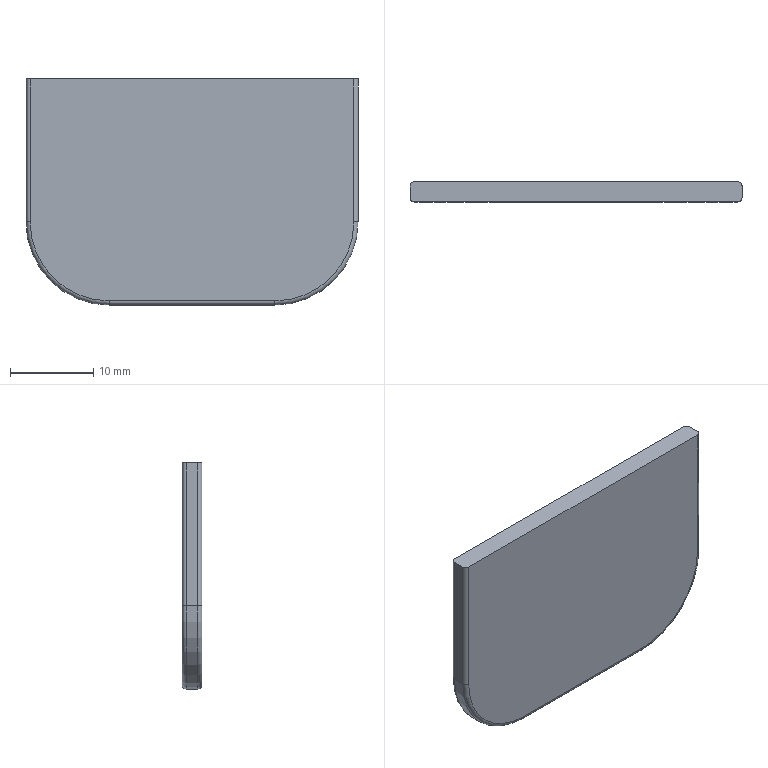Part | STEP file | 1 solid | 18 faces | box 39.94 x 2.4 x 27.2 mm | volume 2495 mm3 | cylinder 8 | plane 6 | torus 4 | commonest cylinder face diameters 1 x6 20 x2
STEP:
#1=CARTESIAN_POINT('',(0.,0.,0.));
#2=DIRECTION('',(0.,0.,1.));
#3=DIRECTION('',(1.,0.,0.));
#4=AXIS2_PLACEMENT_3D('',#1,#2,#3);
#5=CARTESIAN_POINT('',(1352.247,433.78,23.879));
#6=VERTEX_POINT('',#5);
#7=CARTESIAN_POINT('',(1352.247,435.18,23.879));
#8=VERTEX_POINT('',#7);
#9=CARTESIAN_POINT('',(1352.247,-3550.289,23.879));
#10=DIRECTION('',(0.,1.,0.));
#11=VECTOR('',#10,1.);
#12=LINE('',#9,#11);
#13=CARTESIAN_POINT('',(1352.247,433.23,0.979));
#14=DIRECTION('',(1.,0.,0.));
#15=DIRECTION('',(0.,0.,-1.));
#16=AXIS2_PLACEMENT_3D('',#13,#14,#15);
#17=PLANE('',#16);
#18=CARTESIAN_POINT('',(-22.9,-3983.519));
#19=DIRECTION('',(0.,1.));
#20=VECTOR('',#19,1.);
#21=LINE('',#18,#20);
#22=(GEOMETRIC_REPRESENTATION_CONTEXT(2)PARAMETRIC_REPRESENTATION_CONTEXT()REPRESENTATION_CONTEXT('',''));
#23=DEFINITIONAL_REPRESENTATION('',(#21),#22);
#24=PCURVE('',#17,#23);
#25=CARTESIAN_POINT('',(18395.161,-3550.289,23.879));
#26=DIRECTION('',(0.,0.,1.));
#27=DIRECTION('',(1.,0.,0.));
#28=AXIS2_PLACEMENT_3D('',#25,#26,#27);
#29=PLANE('',#28);
#30=CARTESIAN_POINT('',(-17042.914,0.));
#31=DIRECTION('',(0.,1.));
#32=VECTOR('',#31,1.);
#33=LINE('',#30,#32);
#34=(GEOMETRIC_REPRESENTATION_CONTEXT(2)PARAMETRIC_REPRESENTATION_CONTEXT()REPRESENTATION_CONTEXT('',''));
#35=DEFINITIONAL_REPRESENTATION('',(#33),#34);
#36=PCURVE('',#29,#35);
#37=SURFACE_CURVE('',#12,(#24,#36),.PCURVE_S1.);
#38=EDGE_CURVE('',#6,#8,#37,.T.);
#39=ORIENTED_EDGE('',*,*,#38,.F.);
#40=CARTESIAN_POINT('',(1352.247,433.78,6.679));
#41=VERTEX_POINT('',#40);
#42=CARTESIAN_POINT('',(1352.247,433.78,0.979));
#43=DIRECTION('',(0.,0.,-1.));
#44=VECTOR('',#43,1.);
#45=LINE('',#42,#44);
#46=CARTESIAN_POINT('',(0.,0.55));
#47=DIRECTION('',(1.,0.));
#48=VECTOR('',#47,1.);
#49=LINE('',#46,#48);
#50=(GEOMETRIC_REPRESENTATION_CONTEXT(2)PARAMETRIC_REPRESENTATION_CONTEXT()REPRESENTATION_CONTEXT('',''));
#51=DEFINITIONAL_REPRESENTATION('',(#49),#50);
#52=PCURVE('',#17,#51);
#53=CARTESIAN_POINT('',(1351.747,433.78,0.979));
#54=DIRECTION('',(0.,0.,1.));
#55=DIRECTION('',(1.,0.,0.));
#56=AXIS2_PLACEMENT_3D('',#53,#54,#55);
#57=CYLINDRICAL_SURFACE('',#56,0.5);
#58=CARTESIAN_POINT('',(6.283,0.));
#59=DIRECTION('',(0.,-1.));
#60=VECTOR('',#59,1.);
#61=LINE('',#58,#60);
#62=(GEOMETRIC_REPRESENTATION_CONTEXT(2)PARAMETRIC_REPRESENTATION_CONTEXT()REPRESENTATION_CONTEXT('',''));
#63=DEFINITIONAL_REPRESENTATION('',(#61),#62);
#64=PCURVE('',#57,#63);
#65=SURFACE_CURVE('',#45,(#52,#64),.PCURVE_S1.);
#66=EDGE_CURVE('',#6,#41,#65,.T.);
#67=ORIENTED_EDGE('',*,*,#66,.T.);
#68=CARTESIAN_POINT('',(1352.247,435.18,6.679));
#69=VERTEX_POINT('',#68);
#70=CARTESIAN_POINT('',(1352.247,435.68,6.679));
#71=DIRECTION('',(0.,1.,0.));
#72=VECTOR('',#71,1.);
#73=LINE('',#70,#72);
#74=CARTESIAN_POINT('',(-5.7,2.45));
#75=DIRECTION('',(0.,1.));
#76=VECTOR('',#75,1.);
#77=LINE('',#74,#76);
#78=(GEOMETRIC_REPRESENTATION_CONTEXT(2)PARAMETRIC_REPRESENTATION_CONTEXT()REPRESENTATION_CONTEXT('',''));
#79=DEFINITIONAL_REPRESENTATION('',(#77),#78);
#80=PCURVE('',#17,#79);
#81=CARTESIAN_POINT('',(1342.247,433.23,6.679));
#82=DIRECTION('',(0.,1.,0.));
#83=DIRECTION('',(0.,0.,-1.));
#84=AXIS2_PLACEMENT_3D('',#81,#82,#83);
#85=CYLINDRICAL_SURFACE('',#84,10.);
#86=CARTESIAN_POINT('',(4.712,2.45));
#87=DIRECTION('',(0.,1.));
#88=VECTOR('',#87,1.);
#89=LINE('',#86,#88);
#90=(GEOMETRIC_REPRESENTATION_CONTEXT(2)PARAMETRIC_REPRESENTATION_CONTEXT()REPRESENTATION_CONTEXT('',''));
#91=DEFINITIONAL_REPRESENTATION('',(#89),#90);
#92=PCURVE('',#85,#91);
#93=SURFACE_CURVE('',#73,(#80,#92),.PCURVE_S1.);
#94=EDGE_CURVE('',#41,#69,#93,.T.);
#95=ORIENTED_EDGE('',*,*,#94,.T.);
#96=CARTESIAN_POINT('',(1352.247,435.18,0.979));
#97=DIRECTION('',(0.,0.,1.));
#98=VECTOR('',#97,1.);
#99=LINE('',#96,#98);
#100=CARTESIAN_POINT('',(0.,1.95));
#101=DIRECTION('',(-1.,0.));
#102=VECTOR('',#101,1.);
#103=LINE('',#100,#102);
#104=(GEOMETRIC_REPRESENTATION_CONTEXT(2)PARAMETRIC_REPRESENTATION_CONTEXT()REPRESENTATION_CONTEXT('',''));
#105=DEFINITIONAL_REPRESENTATION('',(#103),#104);
#106=PCURVE('',#17,#105);
#107=CARTESIAN_POINT('',(1351.747,435.18,0.979));
#108=DIRECTION('',(0.,0.,1.));
#109=DIRECTION('',(1.,0.,0.));
#110=AXIS2_PLACEMENT_3D('',#107,#108,#109);
#111=CYLINDRICAL_SURFACE('',#110,0.5);
#112=CARTESIAN_POINT('',(0.,0.));
#113=DIRECTION('',(0.,1.));
#114=VECTOR('',#113,1.);
#115=LINE('',#112,#114);
#116=(GEOMETRIC_REPRESENTATION_CONTEXT(2)PARAMETRIC_REPRESENTATION_CONTEXT()REPRESENTATION_CONTEXT('',''));
#117=DEFINITIONAL_REPRESENTATION('',(#115),#116);
#118=PCURVE('',#111,#117);
#119=SURFACE_CURVE('',#99,(#106,#118),.PCURVE_S1.);
#120=EDGE_CURVE('',#69,#8,#119,.T.);
#121=ORIENTED_EDGE('',*,*,#120,.T.);
#122=EDGE_LOOP('',(#39,#67,#95,#121));
#123=FACE_BOUND('',#122,.T.);
#124=ADVANCED_FACE('',(#123),#17,.T.);
#125=CARTESIAN_POINT('',(1351.747,435.68,23.879));
#126=VERTEX_POINT('',#125);
#127=CARTESIAN_POINT('',(1312.807,435.68,23.879));
#128=VERTEX_POINT('',#127);
#129=CARTESIAN_POINT('',(18395.161,435.68,23.879));
#130=DIRECTION('',(-1.,0.,0.));
#131=VECTOR('',#130,1.);
#132=LINE('',#129,#131);
#133=CARTESIAN_POINT('',(1352.277,435.68,0.979));
#134=DIRECTION('',(0.,1.,0.));
#135=DIRECTION('',(0.,0.,-1.));
#136=AXIS2_PLACEMENT_3D('',#133,#134,#135);
#137=PLANE('',#136);
#138=CARTESIAN_POINT('',(-22.9,-17042.884));
#139=DIRECTION('',(0.,1.));
#140=VECTOR('',#139,1.);
#141=LINE('',#138,#140);
#142=(GEOMETRIC_REPRESENTATION_CONTEXT(2)PARAMETRIC_REPRESENTATION_CONTEXT()REPRESENTATION_CONTEXT('',''));
#143=DEFINITIONAL_REPRESENTATION('',(#141),#142);
#144=PCURVE('',#137,#143);
#145=CARTESIAN_POINT('',(0.,3985.969));
#146=DIRECTION('',(-1.,0.));
#147=VECTOR('',#146,1.);
#148=LINE('',#145,#147);
#149=(GEOMETRIC_REPRESENTATION_CONTEXT(2)PARAMETRIC_REPRESENTATION_CONTEXT()REPRESENTATION_CONTEXT('',''));
#150=DEFINITIONAL_REPRESENTATION('',(#148),#149);
#151=PCURVE('',#29,#150);
#152=SURFACE_CURVE('',#132,(#144,#151),.PCURVE_S1.);
#153=EDGE_CURVE('',#126,#128,#152,.T.);
#154=ORIENTED_EDGE('',*,*,#153,.F.);
#155=CARTESIAN_POINT('',(1351.747,435.68,6.679));
#156=VERTEX_POINT('',#155);
#157=CARTESIAN_POINT('',(1351.747,435.68,0.979));
#158=DIRECTION('',(0.,0.,-1.));
#159=VECTOR('',#158,1.);
#160=LINE('',#157,#159);
#161=CARTESIAN_POINT('',(0.,0.53));
#162=DIRECTION('',(1.,0.));
#163=VECTOR('',#162,1.);
#164=LINE('',#161,#163);
#165=(GEOMETRIC_REPRESENTATION_CONTEXT(2)PARAMETRIC_REPRESENTATION_CONTEXT()REPRESENTATION_CONTEXT('',''));
#166=DEFINITIONAL_REPRESENTATION('',(#164),#165);
#167=PCURVE('',#137,#166);
#168=CARTESIAN_POINT('',(1.571,0.));
#169=DIRECTION('',(0.,-1.));
#170=VECTOR('',#169,1.);
#171=LINE('',#168,#170);
#172=(GEOMETRIC_REPRESENTATION_CONTEXT(2)PARAMETRIC_REPRESENTATION_CONTEXT()REPRESENTATION_CONTEXT('',''));
#173=DEFINITIONAL_REPRESENTATION('',(#171),#172);
#174=PCURVE('',#111,#173);
#175=SURFACE_CURVE('',#160,(#167,#174),.PCURVE_S1.);
#176=EDGE_CURVE('',#126,#156,#175,.T.);
#177=ORIENTED_EDGE('',*,*,#176,.T.);
#178=CARTESIAN_POINT('',(1342.247,435.68,-2.821));
#179=VERTEX_POINT('',#178);
#180=CARTESIAN_POINT('',(1342.247,435.68,6.679));
#181=DIRECTION('',(0.,1.,0.));
#182=DIRECTION('',(0.,0.,1.));
#183=AXIS2_PLACEMENT_3D('',#180,#181,#182);
#184=CIRCLE('',#183,9.5);
#185=CARTESIAN_POINT('',(-5.7,10.03));
#186=DIRECTION('',(-1.,0.));
#187=AXIS2_PLACEMENT_2D('',#185,#186);
#188=CIRCLE('',#187,9.5);
#189=(GEOMETRIC_REPRESENTATION_CONTEXT(2)PARAMETRIC_REPRESENTATION_CONTEXT()REPRESENTATION_CONTEXT('',''));
#190=DEFINITIONAL_REPRESENTATION('',(#188),#189);
#191=PCURVE('',#137,#190);
#192=CARTESIAN_POINT('',(1342.247,435.18,6.679));
#193=DIRECTION('',(0.,1.,0.));
#194=DIRECTION('',(0.,0.,-1.));
#195=AXIS2_PLACEMENT_3D('',#192,#193,#194);
#196=TOROIDAL_SURFACE('',#195,9.5,0.5);
#197=CARTESIAN_POINT('',(3.142,1.571));
#198=DIRECTION('',(1.,0.));
#199=VECTOR('',#198,1.);
#200=LINE('',#197,#199);
#201=(GEOMETRIC_REPRESENTATION_CONTEXT(2)PARAMETRIC_REPRESENTATION_CONTEXT()REPRESENTATION_CONTEXT('',''));
#202=DEFINITIONAL_REPRESENTATION('',(#200),#201);
#203=PCURVE('',#196,#202);
#204=SURFACE_CURVE('',#184,(#191,#203),.PCURVE_S1.);
#205=EDGE_CURVE('',#156,#179,#204,.T.);
#206=ORIENTED_EDGE('',*,*,#205,.T.);
#207=CARTESIAN_POINT('',(1322.307,435.68,-2.821));
#208=VERTEX_POINT('',#207);
#209=CARTESIAN_POINT('',(1322.307,435.68,-2.821));
#210=DIRECTION('',(-1.,0.,0.));
#211=VECTOR('',#210,1.);
#212=LINE('',#209,#211);
#213=CARTESIAN_POINT('',(3.8,29.97));
#214=DIRECTION('',(0.,1.));
#215=VECTOR('',#214,1.);
#216=LINE('',#213,#215);
#217=(GEOMETRIC_REPRESENTATION_CONTEXT(2)PARAMETRIC_REPRESENTATION_CONTEXT()REPRESENTATION_CONTEXT('',''));
#218=DEFINITIONAL_REPRESENTATION('',(#216),#217);
#219=PCURVE('',#137,#218);
#220=CARTESIAN_POINT('',(1352.277,435.18,-2.821));
#221=DIRECTION('',(-1.,0.,0.));
#222=DIRECTION('',(0.,0.,1.));
#223=AXIS2_PLACEMENT_3D('',#220,#221,#222);
#224=CYLINDRICAL_SURFACE('',#223,0.5);
#225=CARTESIAN_POINT('',(1.571,29.97));
#226=DIRECTION('',(0.,1.));
#227=VECTOR('',#226,1.);
#228=LINE('',#225,#227);
#229=(GEOMETRIC_REPRESENTATION_CONTEXT(2)PARAMETRIC_REPRESENTATION_CONTEXT()REPRESENTATION_CONTEXT('',''));
#230=DEFINITIONAL_REPRESENTATION('',(#228),#229);
#231=PCURVE('',#224,#230);
#232=SURFACE_CURVE('',#212,(#219,#231),.PCURVE_S1.);
#233=EDGE_CURVE('',#179,#208,#232,.T.);
#234=ORIENTED_EDGE('',*,*,#233,.T.);
#235=CARTESIAN_POINT('',(1312.807,435.68,6.679));
#236=VERTEX_POINT('',#235);
#237=CARTESIAN_POINT('',(1322.307,435.68,6.679));
#238=DIRECTION('',(0.,1.,0.));
#239=DIRECTION('',(0.,0.,1.));
#240=AXIS2_PLACEMENT_3D('',#237,#238,#239);
#241=CIRCLE('',#240,9.5);
#242=CARTESIAN_POINT('',(-5.7,29.97));
#243=DIRECTION('',(-1.,0.));
#244=AXIS2_PLACEMENT_2D('',#242,#243);
#245=CIRCLE('',#244,9.5);
#246=(GEOMETRIC_REPRESENTATION_CONTEXT(2)PARAMETRIC_REPRESENTATION_CONTEXT()REPRESENTATION_CONTEXT('',''));
#247=DEFINITIONAL_REPRESENTATION('',(#245),#246);
#248=PCURVE('',#137,#247);
#249=CARTESIAN_POINT('',(1322.307,435.18,6.679));
#250=DIRECTION('',(0.,1.,0.));
#251=DIRECTION('',(0.,0.,-1.));
#252=AXIS2_PLACEMENT_3D('',#249,#250,#251);
#253=TOROIDAL_SURFACE('',#252,9.5,0.5);
#254=CARTESIAN_POINT('',(-3.142,1.571));
#255=DIRECTION('',(1.,0.));
#256=VECTOR('',#255,1.);
#257=LINE('',#254,#256);
#258=(GEOMETRIC_REPRESENTATION_CONTEXT(2)PARAMETRIC_REPRESENTATION_CONTEXT()REPRESENTATION_CONTEXT('',''));
#259=DEFINITIONAL_REPRESENTATION('',(#257),#258);
#260=PCURVE('',#253,#259);
#261=SURFACE_CURVE('',#241,(#248,#260),.PCURVE_S1.);
#262=EDGE_CURVE('',#208,#236,#261,.T.);
#263=ORIENTED_EDGE('',*,*,#262,.T.);
#264=CARTESIAN_POINT('',(1312.807,435.68,0.979));
#265=DIRECTION('',(0.,0.,1.));
#266=VECTOR('',#265,1.);
#267=LINE('',#264,#266);
#268=CARTESIAN_POINT('',(0.,39.47));
#269=DIRECTION('',(-1.,0.));
#270=VECTOR('',#269,1.);
#271=LINE('',#268,#270);
#272=(GEOMETRIC_REPRESENTATION_CONTEXT(2)PARAMETRIC_REPRESENTATION_CONTEXT()REPRESENTATION_CONTEXT('',''));
#273=DEFINITIONAL_REPRESENTATION('',(#271),#272);
#274=PCURVE('',#137,#273);
#275=CARTESIAN_POINT('',(1312.807,435.18,0.979));
#276=DIRECTION('',(0.,0.,1.));
#277=DIRECTION('',(1.,0.,0.));
#278=AXIS2_PLACEMENT_3D('',#275,#276,#277);
#279=CYLINDRICAL_SURFACE('',#278,0.5);
#280=CARTESIAN_POINT('',(1.571,0.));
#281=DIRECTION('',(0.,1.));
#282=VECTOR('',#281,1.);
#283=LINE('',#280,#282);
#284=(GEOMETRIC_REPRESENTATION_CONTEXT(2)PARAMETRIC_REPRESENTATION_CONTEXT()REPRESENTATION_CONTEXT('',''));
#285=DEFINITIONAL_REPRESENTATION('',(#283),#284);
#286=PCURVE('',#279,#285);
#287=SURFACE_CURVE('',#267,(#274,#286),.PCURVE_S1.);
#288=EDGE_CURVE('',#236,#128,#287,.T.);
#289=ORIENTED_EDGE('',*,*,#288,.T.);
#290=EDGE_LOOP('',(#154,#177,#206,#234,#263,#289));
#291=FACE_BOUND('',#290,.T.);
#292=ADVANCED_FACE('',(#291),#137,.T.);
#293=CARTESIAN_POINT('',(1312.307,435.18,6.679));
#294=VERTEX_POINT('',#293);
#295=CARTESIAN_POINT('',(1312.307,433.78,6.679));
#296=VERTEX_POINT('',#295);
#297=CARTESIAN_POINT('',(1312.307,433.28,6.679));
#298=DIRECTION('',(0.,-1.,0.));
#299=VECTOR('',#298,1.);
#300=LINE('',#297,#299);
#301=CARTESIAN_POINT('',(1312.307,435.73,0.979));
#302=DIRECTION('',(-1.,0.,0.));
#303=DIRECTION('',(0.,0.,1.));
#304=AXIS2_PLACEMENT_3D('',#301,#302,#303);
#305=PLANE('',#304);
#306=CARTESIAN_POINT('',(5.7,-2.45));
#307=DIRECTION('',(0.,-1.));
#308=VECTOR('',#307,1.);
#309=LINE('',#306,#308);
#310=(GEOMETRIC_REPRESENTATION_CONTEXT(2)PARAMETRIC_REPRESENTATION_CONTEXT()REPRESENTATION_CONTEXT('',''));
#311=DEFINITIONAL_REPRESENTATION('',(#309),#310);
#312=PCURVE('',#305,#311);
#313=CARTESIAN_POINT('',(1322.307,435.73,6.679));
#314=DIRECTION('',(0.,-1.,0.));
#315=DIRECTION('',(0.,0.,1.));
#316=AXIS2_PLACEMENT_3D('',#313,#314,#315);
#317=CYLINDRICAL_SURFACE('',#316,10.);
#318=CARTESIAN_POINT('',(1.571,2.45));
#319=DIRECTION('',(0.,1.));
#320=VECTOR('',#319,1.);
#321=LINE('',#318,#320);
#322=(GEOMETRIC_REPRESENTATION_CONTEXT(2)PARAMETRIC_REPRESENTATION_CONTEXT()REPRESENTATION_CONTEXT('',''));
#323=DEFINITIONAL_REPRESENTATION('',(#321),#322);
#324=PCURVE('',#317,#323);
#325=SURFACE_CURVE('',#300,(#312,#324),.PCURVE_S1.);
#326=EDGE_CURVE('',#294,#296,#325,.T.);
#327=ORIENTED_EDGE('',*,*,#326,.T.);
#328=CARTESIAN_POINT('',(1312.307,433.78,23.879));
#329=VERTEX_POINT('',#328);
#330=CARTESIAN_POINT('',(1312.307,433.78,0.979));
#331=DIRECTION('',(0.,0.,1.));
#332=VECTOR('',#331,1.);
#333=LINE('',#330,#332);
#334=CARTESIAN_POINT('',(0.,-1.95));
#335=DIRECTION('',(1.,0.));
#336=VECTOR('',#335,1.);
#337=LINE('',#334,#336);
#338=(GEOMETRIC_REPRESENTATION_CONTEXT(2)PARAMETRIC_REPRESENTATION_CONTEXT()REPRESENTATION_CONTEXT('',''));
#339=DEFINITIONAL_REPRESENTATION('',(#337),#338);
#340=PCURVE('',#305,#339);
#341=CARTESIAN_POINT('',(1312.807,433.78,0.979));
#342=DIRECTION('',(0.,0.,1.));
#343=DIRECTION('',(1.,0.,0.));
#344=AXIS2_PLACEMENT_3D('',#341,#342,#343);
#345=CYLINDRICAL_SURFACE('',#344,0.5);
#346=CARTESIAN_POINT('',(3.142,0.));
#347=DIRECTION('',(0.,1.));
#348=VECTOR('',#347,1.);
#349=LINE('',#346,#348);
#350=(GEOMETRIC_REPRESENTATION_CONTEXT(2)PARAMETRIC_REPRESENTATION_CONTEXT()REPRESENTATION_CONTEXT('',''));
#351=DEFINITIONAL_REPRESENTATION('',(#349),#350);
#352=PCURVE('',#345,#351);
#353=SURFACE_CURVE('',#333,(#340,#352),.PCURVE_S1.);
#354=EDGE_CURVE('',#296,#329,#353,.T.);
#355=ORIENTED_EDGE('',*,*,#354,.T.);
#356=CARTESIAN_POINT('',(1312.307,435.18,23.879));
#357=VERTEX_POINT('',#356);
#358=CARTESIAN_POINT('',(1312.307,-3550.289,23.879));
#359=DIRECTION('',(0.,-1.,0.));
#360=VECTOR('',#359,1.);
#361=LINE('',#358,#360);
#362=CARTESIAN_POINT('',(22.9,-3986.019));
#363=DIRECTION('',(0.,-1.));
#364=VECTOR('',#363,1.);
#365=LINE('',#362,#364);
#366=(GEOMETRIC_REPRESENTATION_CONTEXT(2)PARAMETRIC_REPRESENTATION_CONTEXT()REPRESENTATION_CONTEXT('',''));
#367=DEFINITIONAL_REPRESENTATION('',(#365),#366);
#368=PCURVE('',#305,#367);
#369=CARTESIAN_POINT('',(-17082.854,0.));
#370=DIRECTION('',(0.,-1.));
#371=VECTOR('',#370,1.);
#372=LINE('',#369,#371);
#373=(GEOMETRIC_REPRESENTATION_CONTEXT(2)PARAMETRIC_REPRESENTATION_CONTEXT()REPRESENTATION_CONTEXT('',''));
#374=DEFINITIONAL_REPRESENTATION('',(#372),#373);
#375=PCURVE('',#29,#374);
#376=SURFACE_CURVE('',#361,(#368,#375),.PCURVE_S1.);
#377=EDGE_CURVE('',#357,#329,#376,.T.);
#378=ORIENTED_EDGE('',*,*,#377,.F.);
#379=CARTESIAN_POINT('',(1312.307,435.18,0.979));
#380=DIRECTION('',(0.,0.,-1.));
#381=VECTOR('',#380,1.);
#382=LINE('',#379,#381);
#383=CARTESIAN_POINT('',(0.,-0.55));
#384=DIRECTION('',(-1.,0.));
#385=VECTOR('',#384,1.);
#386=LINE('',#383,#385);
#387=(GEOMETRIC_REPRESENTATION_CONTEXT(2)PARAMETRIC_REPRESENTATION_CONTEXT()REPRESENTATION_CONTEXT('',''));
#388=DEFINITIONAL_REPRESENTATION('',(#386),#387);
#389=PCURVE('',#305,#388);
#390=CARTESIAN_POINT('',(3.142,0.));
#391=DIRECTION('',(0.,-1.));
#392=VECTOR('',#391,1.);
#393=LINE('',#390,#392);
#394=(GEOMETRIC_REPRESENTATION_CONTEXT(2)PARAMETRIC_REPRESENTATION_CONTEXT()REPRESENTATION_CONTEXT('',''));
#395=DEFINITIONAL_REPRESENTATION('',(#393),#394);
#396=PCURVE('',#279,#395);
#397=SURFACE_CURVE('',#382,(#389,#396),.PCURVE_S1.);
#398=EDGE_CURVE('',#357,#294,#397,.T.);
#399=ORIENTED_EDGE('',*,*,#398,.T.);
#400=EDGE_LOOP('',(#327,#355,#378,#399));
#401=FACE_BOUND('',#400,.T.);
#402=ADVANCED_FACE('',(#401),#305,.T.);
#403=CARTESIAN_POINT('',(1312.807,433.28,23.879));
#404=VERTEX_POINT('',#403);
#405=CARTESIAN_POINT('',(1351.747,433.28,23.879));
#406=VERTEX_POINT('',#405);
#407=CARTESIAN_POINT('',(18395.161,433.28,23.879));
#408=DIRECTION('',(1.,0.,0.));
#409=VECTOR('',#408,1.);
#410=LINE('',#407,#409);
#411=CARTESIAN_POINT('',(1312.277,433.28,0.979));
#412=DIRECTION('',(0.,-1.,0.));
#413=DIRECTION('',(0.,0.,1.));
#414=AXIS2_PLACEMENT_3D('',#411,#412,#413);
#415=PLANE('',#414);
#416=CARTESIAN_POINT('',(22.9,-17082.884));
#417=DIRECTION('',(0.,-1.));
#418=VECTOR('',#417,1.);
#419=LINE('',#416,#418);
#420=(GEOMETRIC_REPRESENTATION_CONTEXT(2)PARAMETRIC_REPRESENTATION_CONTEXT()REPRESENTATION_CONTEXT('',''));
#421=DEFINITIONAL_REPRESENTATION('',(#419),#420);
#422=PCURVE('',#415,#421);
#423=CARTESIAN_POINT('',(0.,3983.569));
#424=DIRECTION('',(1.,0.));
#425=VECTOR('',#424,1.);
#426=LINE('',#423,#425);
#427=(GEOMETRIC_REPRESENTATION_CONTEXT(2)PARAMETRIC_REPRESENTATION_CONTEXT()REPRESENTATION_CONTEXT('',''));
#428=DEFINITIONAL_REPRESENTATION('',(#426),#427);
#429=PCURVE('',#29,#428);
#430=SURFACE_CURVE('',#410,(#422,#429),.PCURVE_S1.);
#431=EDGE_CURVE('',#404,#406,#430,.T.);
#432=ORIENTED_EDGE('',*,*,#431,.F.);
#433=CARTESIAN_POINT('',(1312.807,433.28,6.679));
#434=VERTEX_POINT('',#433);
#435=CARTESIAN_POINT('',(1312.807,433.28,0.979));
#436=DIRECTION('',(0.,0.,-1.));
#437=VECTOR('',#436,1.);
#438=LINE('',#435,#437);
#439=CARTESIAN_POINT('',(0.,-0.53));
#440=DIRECTION('',(-1.,0.));
#441=VECTOR('',#440,1.);
#442=LINE('',#439,#441);
#443=(GEOMETRIC_REPRESENTATION_CONTEXT(2)PARAMETRIC_REPRESENTATION_CONTEXT()REPRESENTATION_CONTEXT('',''));
#444=DEFINITIONAL_REPRESENTATION('',(#442),#443);
#445=PCURVE('',#415,#444);
#446=CARTESIAN_POINT('',(4.712,0.));
#447=DIRECTION('',(0.,-1.));
#448=VECTOR('',#447,1.);
#449=LINE('',#446,#448);
#450=(GEOMETRIC_REPRESENTATION_CONTEXT(2)PARAMETRIC_REPRESENTATION_CONTEXT()REPRESENTATION_CONTEXT('',''));
#451=DEFINITIONAL_REPRESENTATION('',(#449),#450);
#452=PCURVE('',#345,#451);
#453=SURFACE_CURVE('',#438,(#445,#452),.PCURVE_S1.);
#454=EDGE_CURVE('',#404,#434,#453,.T.);
#455=ORIENTED_EDGE('',*,*,#454,.T.);
#456=CARTESIAN_POINT('',(1322.307,433.28,-2.821));
#457=VERTEX_POINT('',#456);
#458=CARTESIAN_POINT('',(1322.307,433.28,6.679));
#459=DIRECTION('',(0.,-1.,0.));
#460=DIRECTION('',(0.,0.,-1.));
#461=AXIS2_PLACEMENT_3D('',#458,#459,#460);
#462=CIRCLE('',#461,9.5);
#463=CARTESIAN_POINT('',(5.7,-10.03));
#464=DIRECTION('',(-1.,0.));
#465=AXIS2_PLACEMENT_2D('',#463,#464);
#466=CIRCLE('',#465,9.5);
#467=(GEOMETRIC_REPRESENTATION_CONTEXT(2)PARAMETRIC_REPRESENTATION_CONTEXT()REPRESENTATION_CONTEXT('',''));
#468=DEFINITIONAL_REPRESENTATION('',(#466),#467);
#469=PCURVE('',#415,#468);
#470=CARTESIAN_POINT('',(1322.307,433.78,6.679));
#471=DIRECTION('',(0.,-1.,0.));
#472=DIRECTION('',(0.,0.,1.));
#473=AXIS2_PLACEMENT_3D('',#470,#471,#472);
#474=TOROIDAL_SURFACE('',#473,9.5,0.5);
#475=CARTESIAN_POINT('',(-3.142,1.571));
#476=DIRECTION('',(1.,0.));
#477=VECTOR('',#476,1.);
#478=LINE('',#475,#477);
#479=(GEOMETRIC_REPRESENTATION_CONTEXT(2)PARAMETRIC_REPRESENTATION_CONTEXT()REPRESENTATION_CONTEXT('',''));
#480=DEFINITIONAL_REPRESENTATION('',(#478),#479);
#481=PCURVE('',#474,#480);
#482=SURFACE_CURVE('',#462,(#469,#481),.PCURVE_S1.);
#483=EDGE_CURVE('',#434,#457,#482,.T.);
#484=ORIENTED_EDGE('',*,*,#483,.T.);
#485=CARTESIAN_POINT('',(1342.247,433.28,-2.821));
#486=VERTEX_POINT('',#485);
#487=CARTESIAN_POINT('',(1342.247,433.28,-2.821));
#488=DIRECTION('',(1.,0.,0.));
#489=VECTOR('',#488,1.);
#490=LINE('',#487,#489);
#491=CARTESIAN_POINT('',(-3.8,-29.97));
#492=DIRECTION('',(0.,-1.));
#493=VECTOR('',#492,1.);
#494=LINE('',#491,#493);
#495=(GEOMETRIC_REPRESENTATION_CONTEXT(2)PARAMETRIC_REPRESENTATION_CONTEXT()REPRESENTATION_CONTEXT('',''));
#496=DEFINITIONAL_REPRESENTATION('',(#494),#495);
#497=PCURVE('',#415,#496);
#498=CARTESIAN_POINT('',(1312.277,433.78,-2.821));
#499=DIRECTION('',(1.,0.,0.));
#500=DIRECTION('',(0.,0.,-1.));
#501=AXIS2_PLACEMENT_3D('',#498,#499,#500);
#502=CYLINDRICAL_SURFACE('',#501,0.5);
#503=CARTESIAN_POINT('',(4.712,29.97));
#504=DIRECTION('',(0.,1.));
#505=VECTOR('',#504,1.);
#506=LINE('',#503,#505);
#507=(GEOMETRIC_REPRESENTATION_CONTEXT(2)PARAMETRIC_REPRESENTATION_CONTEXT()REPRESENTATION_CONTEXT('',''));
#508=DEFINITIONAL_REPRESENTATION('',(#506),#507);
#509=PCURVE('',#502,#508);
#510=SURFACE_CURVE('',#490,(#497,#509),.PCURVE_S1.);
#511=EDGE_CURVE('',#457,#486,#510,.T.);
#512=ORIENTED_EDGE('',*,*,#511,.T.);
#513=CARTESIAN_POINT('',(1351.747,433.28,6.679));
#514=VERTEX_POINT('',#513);
#515=CARTESIAN_POINT('',(1342.247,433.28,6.679));
#516=DIRECTION('',(0.,-1.,0.));
#517=DIRECTION('',(0.,0.,-1.));
#518=AXIS2_PLACEMENT_3D('',#515,#516,#517);
#519=CIRCLE('',#518,9.5);
#520=CARTESIAN_POINT('',(5.7,-29.97));
#521=DIRECTION('',(-1.,0.));
#522=AXIS2_PLACEMENT_2D('',#520,#521);
#523=CIRCLE('',#522,9.5);
#524=(GEOMETRIC_REPRESENTATION_CONTEXT(2)PARAMETRIC_REPRESENTATION_CONTEXT()REPRESENTATION_CONTEXT('',''));
#525=DEFINITIONAL_REPRESENTATION('',(#523),#524);
#526=PCURVE('',#415,#525);
#527=CARTESIAN_POINT('',(1342.247,433.78,6.679));
#528=DIRECTION('',(0.,-1.,0.));
#529=DIRECTION('',(0.,0.,1.));
#530=AXIS2_PLACEMENT_3D('',#527,#528,#529);
#531=TOROIDAL_SURFACE('',#530,9.5,0.5);
#532=CARTESIAN_POINT('',(3.142,1.571));
#533=DIRECTION('',(1.,0.));
#534=VECTOR('',#533,1.);
#535=LINE('',#532,#534);
#536=(GEOMETRIC_REPRESENTATION_CONTEXT(2)PARAMETRIC_REPRESENTATION_CONTEXT()REPRESENTATION_CONTEXT('',''));
#537=DEFINITIONAL_REPRESENTATION('',(#535),#536);
#538=PCURVE('',#531,#537);
#539=SURFACE_CURVE('',#519,(#526,#538),.PCURVE_S1.);
#540=EDGE_CURVE('',#486,#514,#539,.T.);
#541=ORIENTED_EDGE('',*,*,#540,.T.);
#542=CARTESIAN_POINT('',(1351.747,433.28,0.979));
#543=DIRECTION('',(0.,0.,1.));
#544=VECTOR('',#543,1.);
#545=LINE('',#542,#544);
#546=CARTESIAN_POINT('',(0.,-39.47));
#547=DIRECTION('',(1.,0.));
#548=VECTOR('',#547,1.);
#549=LINE('',#546,#548);
#550=(GEOMETRIC_REPRESENTATION_CONTEXT(2)PARAMETRIC_REPRESENTATION_CONTEXT()REPRESENTATION_CONTEXT('',''));
#551=DEFINITIONAL_REPRESENTATION('',(#549),#550);
#552=PCURVE('',#415,#551);
#553=CARTESIAN_POINT('',(4.712,0.));
#554=DIRECTION('',(0.,1.));
#555=VECTOR('',#554,1.);
#556=LINE('',#553,#555);
#557=(GEOMETRIC_REPRESENTATION_CONTEXT(2)PARAMETRIC_REPRESENTATION_CONTEXT()REPRESENTATION_CONTEXT('',''));
#558=DEFINITIONAL_REPRESENTATION('',(#556),#557);
#559=PCURVE('',#57,#558);
#560=SURFACE_CURVE('',#545,(#552,#559),.PCURVE_S1.);
#561=EDGE_CURVE('',#514,#406,#560,.T.);
#562=ORIENTED_EDGE('',*,*,#561,.T.);
#563=EDGE_LOOP('',(#432,#455,#484,#512,#541,#562));
#564=FACE_BOUND('',#563,.T.);
#565=ADVANCED_FACE('',(#564),#415,.T.);
#566=CARTESIAN_POINT('',(1342.247,435.18,-3.321));
#567=VERTEX_POINT('',#566);
#568=CARTESIAN_POINT('',(1342.247,433.78,-3.321));
#569=VERTEX_POINT('',#568);
#570=CARTESIAN_POINT('',(1342.247,433.28,-3.321));
#571=DIRECTION('',(0.,-1.,0.));
#572=VECTOR('',#571,1.);
#573=LINE('',#570,#572);
#574=CARTESIAN_POINT('',(1359.213,511.68,-3.321));
#575=DIRECTION('',(0.,0.,-1.));
#576=DIRECTION('',(-1.,0.,0.));
#577=AXIS2_PLACEMENT_3D('',#574,#575,#576);
#578=PLANE('',#577);
#579=CARTESIAN_POINT('',(16.966,-78.4));
#580=DIRECTION('',(0.,-1.));
#581=VECTOR('',#580,1.);
#582=LINE('',#579,#581);
#583=(GEOMETRIC_REPRESENTATION_CONTEXT(2)PARAMETRIC_REPRESENTATION_CONTEXT()REPRESENTATION_CONTEXT('',''));
#584=DEFINITIONAL_REPRESENTATION('',(#582),#583);
#585=PCURVE('',#578,#584);
#586=CARTESIAN_POINT('',(6.283,0.05));
#587=DIRECTION('',(0.,-1.));
#588=VECTOR('',#587,1.);
#589=LINE('',#586,#588);
#590=(GEOMETRIC_REPRESENTATION_CONTEXT(2)PARAMETRIC_REPRESENTATION_CONTEXT()REPRESENTATION_CONTEXT('',''));
#591=DEFINITIONAL_REPRESENTATION('',(#589),#590);
#592=PCURVE('',#85,#591);
#593=SURFACE_CURVE('',#573,(#585,#592),.PCURVE_S1.);
#594=EDGE_CURVE('',#567,#569,#593,.T.);
#595=ORIENTED_EDGE('',*,*,#594,.T.);
#596=CARTESIAN_POINT('',(1322.307,433.78,-3.321));
#597=VERTEX_POINT('',#596);
#598=CARTESIAN_POINT('',(1322.307,433.78,-3.321));
#599=DIRECTION('',(-1.,0.,0.));
#600=VECTOR('',#599,1.);
#601=LINE('',#598,#600);
#602=CARTESIAN_POINT('',(36.906,-77.9));
#603=DIRECTION('',(1.,0.));
#604=VECTOR('',#603,1.);
#605=LINE('',#602,#604);
#606=(GEOMETRIC_REPRESENTATION_CONTEXT(2)PARAMETRIC_REPRESENTATION_CONTEXT()REPRESENTATION_CONTEXT('',''));
#607=DEFINITIONAL_REPRESENTATION('',(#605),#606);
#608=PCURVE('',#578,#607);
#609=CARTESIAN_POINT('',(6.283,10.03));
#610=DIRECTION('',(0.,-1.));
#611=VECTOR('',#610,1.);
#612=LINE('',#609,#611);
#613=(GEOMETRIC_REPRESENTATION_CONTEXT(2)PARAMETRIC_REPRESENTATION_CONTEXT()REPRESENTATION_CONTEXT('',''));
#614=DEFINITIONAL_REPRESENTATION('',(#612),#613);
#615=PCURVE('',#502,#614);
#616=SURFACE_CURVE('',#601,(#608,#615),.PCURVE_S1.);
#617=EDGE_CURVE('',#569,#597,#616,.T.);
#618=ORIENTED_EDGE('',*,*,#617,.T.);
#619=CARTESIAN_POINT('',(1322.307,435.18,-3.321));
#620=VERTEX_POINT('',#619);
#621=CARTESIAN_POINT('',(1322.307,435.68,-3.321));
#622=DIRECTION('',(0.,1.,0.));
#623=VECTOR('',#622,1.);
#624=LINE('',#621,#623);
#625=CARTESIAN_POINT('',(36.906,-76.));
#626=DIRECTION('',(0.,1.));
#627=VECTOR('',#626,1.);
#628=LINE('',#625,#627);
#629=(GEOMETRIC_REPRESENTATION_CONTEXT(2)PARAMETRIC_REPRESENTATION_CONTEXT()REPRESENTATION_CONTEXT('',''));
#630=DEFINITIONAL_REPRESENTATION('',(#628),#629);
#631=PCURVE('',#578,#630);
#632=CARTESIAN_POINT('',(3.142,0.05));
#633=DIRECTION('',(0.,-1.));
#634=VECTOR('',#633,1.);
#635=LINE('',#632,#634);
#636=(GEOMETRIC_REPRESENTATION_CONTEXT(2)PARAMETRIC_REPRESENTATION_CONTEXT()REPRESENTATION_CONTEXT('',''));
#637=DEFINITIONAL_REPRESENTATION('',(#635),#636);
#638=PCURVE('',#317,#637);
#639=SURFACE_CURVE('',#624,(#631,#638),.PCURVE_S1.);
#640=EDGE_CURVE('',#597,#620,#639,.T.);
#641=ORIENTED_EDGE('',*,*,#640,.T.);
#642=CARTESIAN_POINT('',(1342.247,435.18,-3.321));
#643=DIRECTION('',(1.,0.,0.));
#644=VECTOR('',#643,1.);
#645=LINE('',#642,#644);
#646=CARTESIAN_POINT('',(16.966,-76.5));
#647=DIRECTION('',(-1.,0.));
#648=VECTOR('',#647,1.);
#649=LINE('',#646,#648);
#650=(GEOMETRIC_REPRESENTATION_CONTEXT(2)PARAMETRIC_REPRESENTATION_CONTEXT()REPRESENTATION_CONTEXT('',''));
#651=DEFINITIONAL_REPRESENTATION('',(#649),#650);
#652=PCURVE('',#578,#651);
#653=CARTESIAN_POINT('',(3.142,10.03));
#654=DIRECTION('',(0.,-1.));
#655=VECTOR('',#654,1.);
#656=LINE('',#653,#655);
#657=(GEOMETRIC_REPRESENTATION_CONTEXT(2)PARAMETRIC_REPRESENTATION_CONTEXT()REPRESENTATION_CONTEXT('',''));
#658=DEFINITIONAL_REPRESENTATION('',(#656),#657);
#659=PCURVE('',#224,#658);
#660=SURFACE_CURVE('',#645,(#652,#659),.PCURVE_S1.);
#661=EDGE_CURVE('',#620,#567,#660,.T.);
#662=ORIENTED_EDGE('',*,*,#661,.T.);
#663=EDGE_LOOP('',(#595,#618,#641,#662));
#664=FACE_BOUND('',#663,.T.);
#665=ADVANCED_FACE('',(#664),#578,.T.);
#666=ORIENTED_EDGE('',*,*,#377,.T.);
#667=CARTESIAN_POINT('',(1312.807,433.78,23.879));
#668=DIRECTION('',(0.,0.,1.));
#669=DIRECTION('',(-1.,0.,0.));
#670=AXIS2_PLACEMENT_3D('',#667,#668,#669);
#671=CIRCLE('',#670,0.5);
#672=CARTESIAN_POINT('',(-17082.354,3984.069));
#673=DIRECTION('',(-1.,0.));
#674=AXIS2_PLACEMENT_2D('',#672,#673);
#675=CIRCLE('',#674,0.5);
#676=(GEOMETRIC_REPRESENTATION_CONTEXT(2)PARAMETRIC_REPRESENTATION_CONTEXT()REPRESENTATION_CONTEXT('',''));
#677=DEFINITIONAL_REPRESENTATION('',(#675),#676);
#678=PCURVE('',#29,#677);
#679=CARTESIAN_POINT('',(3.142,22.9));
#680=DIRECTION('',(1.,0.));
#681=VECTOR('',#680,1.);
#682=LINE('',#679,#681);
#683=(GEOMETRIC_REPRESENTATION_CONTEXT(2)PARAMETRIC_REPRESENTATION_CONTEXT()REPRESENTATION_CONTEXT('',''));
#684=DEFINITIONAL_REPRESENTATION('',(#682),#683);
#685=PCURVE('',#345,#684);
#686=SURFACE_CURVE('',#671,(#678,#685),.PCURVE_S1.);
#687=EDGE_CURVE('',#329,#404,#686,.T.);
#688=ORIENTED_EDGE('',*,*,#687,.T.);
#689=ORIENTED_EDGE('',*,*,#431,.T.);
#690=CARTESIAN_POINT('',(1351.747,433.78,23.879));
#691=DIRECTION('',(0.,0.,1.));
#692=DIRECTION('',(-1.,0.,0.));
#693=AXIS2_PLACEMENT_3D('',#690,#691,#692);
#694=CIRCLE('',#693,0.5);
#695=CARTESIAN_POINT('',(-17043.414,3984.069));
#696=DIRECTION('',(-1.,0.));
#697=AXIS2_PLACEMENT_2D('',#695,#696);
#698=CIRCLE('',#697,0.5);
#699=(GEOMETRIC_REPRESENTATION_CONTEXT(2)PARAMETRIC_REPRESENTATION_CONTEXT()REPRESENTATION_CONTEXT('',''));
#700=DEFINITIONAL_REPRESENTATION('',(#698),#699);
#701=PCURVE('',#29,#700);
#702=CARTESIAN_POINT('',(3.142,22.9));
#703=DIRECTION('',(1.,0.));
#704=VECTOR('',#703,1.);
#705=LINE('',#702,#704);
#706=(GEOMETRIC_REPRESENTATION_CONTEXT(2)PARAMETRIC_REPRESENTATION_CONTEXT()REPRESENTATION_CONTEXT('',''));
#707=DEFINITIONAL_REPRESENTATION('',(#705),#706);
#708=PCURVE('',#57,#707);
#709=SURFACE_CURVE('',#694,(#701,#708),.PCURVE_S1.);
#710=EDGE_CURVE('',#406,#6,#709,.T.);
#711=ORIENTED_EDGE('',*,*,#710,.T.);
#712=ORIENTED_EDGE('',*,*,#38,.T.);
#713=CARTESIAN_POINT('',(1351.747,435.18,23.879));
#714=DIRECTION('',(0.,0.,1.));
#715=DIRECTION('',(-1.,0.,0.));
#716=AXIS2_PLACEMENT_3D('',#713,#714,#715);
#717=CIRCLE('',#716,0.5);
#718=CARTESIAN_POINT('',(-17043.414,3985.469));
#719=DIRECTION('',(-1.,0.));
#720=AXIS2_PLACEMENT_2D('',#718,#719);
#721=CIRCLE('',#720,0.5);
#722=(GEOMETRIC_REPRESENTATION_CONTEXT(2)PARAMETRIC_REPRESENTATION_CONTEXT()REPRESENTATION_CONTEXT('',''));
#723=DEFINITIONAL_REPRESENTATION('',(#721),#722);
#724=PCURVE('',#29,#723);
#725=CARTESIAN_POINT('',(-3.142,22.9));
#726=DIRECTION('',(1.,0.));
#727=VECTOR('',#726,1.);
#728=LINE('',#725,#727);
#729=(GEOMETRIC_REPRESENTATION_CONTEXT(2)PARAMETRIC_REPRESENTATION_CONTEXT()REPRESENTATION_CONTEXT('',''));
#730=DEFINITIONAL_REPRESENTATION('',(#728),#729);
#731=PCURVE('',#111,#730);
#732=SURFACE_CURVE('',#717,(#724,#731),.PCURVE_S1.);
#733=EDGE_CURVE('',#8,#126,#732,.T.);
#734=ORIENTED_EDGE('',*,*,#733,.T.);
#735=ORIENTED_EDGE('',*,*,#153,.T.);
#736=CARTESIAN_POINT('',(1312.807,435.18,23.879));
#737=DIRECTION('',(0.,0.,1.));
#738=DIRECTION('',(-1.,0.,0.));
#739=AXIS2_PLACEMENT_3D('',#736,#737,#738);
#740=CIRCLE('',#739,0.5);
#741=CARTESIAN_POINT('',(-17082.354,3985.469));
#742=DIRECTION('',(-1.,0.));
#743=AXIS2_PLACEMENT_2D('',#741,#742);
#744=CIRCLE('',#743,0.5);
#745=(GEOMETRIC_REPRESENTATION_CONTEXT(2)PARAMETRIC_REPRESENTATION_CONTEXT()REPRESENTATION_CONTEXT('',''));
#746=DEFINITIONAL_REPRESENTATION('',(#744),#745);
#747=PCURVE('',#29,#746);
#748=CARTESIAN_POINT('',(-3.142,22.9));
#749=DIRECTION('',(1.,0.));
#750=VECTOR('',#749,1.);
#751=LINE('',#748,#750);
#752=(GEOMETRIC_REPRESENTATION_CONTEXT(2)PARAMETRIC_REPRESENTATION_CONTEXT()REPRESENTATION_CONTEXT('',''));
#753=DEFINITIONAL_REPRESENTATION('',(#751),#752);
#754=PCURVE('',#279,#753);
#755=SURFACE_CURVE('',#740,(#747,#754),.PCURVE_S1.);
#756=EDGE_CURVE('',#128,#357,#755,.T.);
#757=ORIENTED_EDGE('',*,*,#756,.T.);
#758=EDGE_LOOP('',(#666,#688,#689,#711,#712,#734,#735,#757));
#759=FACE_BOUND('',#758,.T.);
#760=ADVANCED_FACE('',(#759),#29,.T.);
#761=ORIENTED_EDGE('',*,*,#640,.F.);
#762=CARTESIAN_POINT('',(1322.307,433.78,6.679));
#763=DIRECTION('',(0.,1.,0.));
#764=DIRECTION('',(0.,0.,-1.));
#765=AXIS2_PLACEMENT_3D('',#762,#763,#764);
#766=CIRCLE('',#765,10.);
#767=CARTESIAN_POINT('',(3.142,1.95));
#768=DIRECTION('',(-1.,0.));
#769=VECTOR('',#768,1.);
#770=LINE('',#767,#769);
#771=(GEOMETRIC_REPRESENTATION_CONTEXT(2)PARAMETRIC_REPRESENTATION_CONTEXT()REPRESENTATION_CONTEXT('',''));
#772=DEFINITIONAL_REPRESENTATION('',(#770),#771);
#773=PCURVE('',#317,#772);
#774=CARTESIAN_POINT('',(3.142,0.));
#775=DIRECTION('',(-1.,0.));
#776=VECTOR('',#775,1.);
#777=LINE('',#774,#776);
#778=(GEOMETRIC_REPRESENTATION_CONTEXT(2)PARAMETRIC_REPRESENTATION_CONTEXT()REPRESENTATION_CONTEXT('',''));
#779=DEFINITIONAL_REPRESENTATION('',(#777),#778);
#780=PCURVE('',#474,#779);
#781=SURFACE_CURVE('',#766,(#773,#780),.PCURVE_S1.);
#782=EDGE_CURVE('',#597,#296,#781,.T.);
#783=ORIENTED_EDGE('',*,*,#782,.T.);
#784=ORIENTED_EDGE('',*,*,#326,.F.);
#785=CARTESIAN_POINT('',(1322.307,435.18,6.679));
#786=DIRECTION('',(0.,-1.,0.));
#787=DIRECTION('',(0.,0.,1.));
#788=AXIS2_PLACEMENT_3D('',#785,#786,#787);
#789=CIRCLE('',#788,10.);
#790=CARTESIAN_POINT('',(0.,0.55));
#791=DIRECTION('',(1.,0.));
#792=VECTOR('',#791,1.);
#793=LINE('',#790,#792);
#794=(GEOMETRIC_REPRESENTATION_CONTEXT(2)PARAMETRIC_REPRESENTATION_CONTEXT()REPRESENTATION_CONTEXT('',''));
#795=DEFINITIONAL_REPRESENTATION('',(#793),#794);
#796=PCURVE('',#317,#795);
#797=CARTESIAN_POINT('',(3.142,0.));
#798=DIRECTION('',(-1.,0.));
#799=VECTOR('',#798,1.);
#800=LINE('',#797,#799);
#801=(GEOMETRIC_REPRESENTATION_CONTEXT(2)PARAMETRIC_REPRESENTATION_CONTEXT()REPRESENTATION_CONTEXT('',''));
#802=DEFINITIONAL_REPRESENTATION('',(#800),#801);
#803=PCURVE('',#253,#802);
#804=SURFACE_CURVE('',#789,(#796,#803),.PCURVE_S1.);
#805=EDGE_CURVE('',#294,#620,#804,.T.);
#806=ORIENTED_EDGE('',*,*,#805,.T.);
#807=EDGE_LOOP('',(#761,#783,#784,#806));
#808=FACE_BOUND('',#807,.T.);
#809=ADVANCED_FACE('',(#808),#317,.T.);
#810=ORIENTED_EDGE('',*,*,#94,.F.);
#811=CARTESIAN_POINT('',(1342.247,433.78,6.679));
#812=DIRECTION('',(0.,1.,0.));
#813=DIRECTION('',(0.,0.,-1.));
#814=AXIS2_PLACEMENT_3D('',#811,#812,#813);
#815=CIRCLE('',#814,10.);
#816=CARTESIAN_POINT('',(0.,0.55));
#817=DIRECTION('',(1.,0.));
#818=VECTOR('',#817,1.);
#819=LINE('',#816,#818);
#820=(GEOMETRIC_REPRESENTATION_CONTEXT(2)PARAMETRIC_REPRESENTATION_CONTEXT()REPRESENTATION_CONTEXT('',''));
#821=DEFINITIONAL_REPRESENTATION('',(#819),#820);
#822=PCURVE('',#85,#821);
#823=CARTESIAN_POINT('',(9.425,0.));
#824=DIRECTION('',(-1.,0.));
#825=VECTOR('',#824,1.);
#826=LINE('',#823,#825);
#827=(GEOMETRIC_REPRESENTATION_CONTEXT(2)PARAMETRIC_REPRESENTATION_CONTEXT()REPRESENTATION_CONTEXT('',''));
#828=DEFINITIONAL_REPRESENTATION('',(#826),#827);
#829=PCURVE('',#531,#828);
#830=SURFACE_CURVE('',#815,(#822,#829),.PCURVE_S1.);
#831=EDGE_CURVE('',#41,#569,#830,.T.);
#832=ORIENTED_EDGE('',*,*,#831,.T.);
#833=ORIENTED_EDGE('',*,*,#594,.F.);
#834=CARTESIAN_POINT('',(1342.247,435.18,6.679));
#835=DIRECTION('',(0.,-1.,0.));
#836=DIRECTION('',(0.,0.,1.));
#837=AXIS2_PLACEMENT_3D('',#834,#835,#836);
#838=CIRCLE('',#837,10.);
#839=CARTESIAN_POINT('',(9.425,1.95));
#840=DIRECTION('',(-1.,0.));
#841=VECTOR('',#840,1.);
#842=LINE('',#839,#841);
#843=(GEOMETRIC_REPRESENTATION_CONTEXT(2)PARAMETRIC_REPRESENTATION_CONTEXT()REPRESENTATION_CONTEXT('',''));
#844=DEFINITIONAL_REPRESENTATION('',(#842),#843);
#845=PCURVE('',#85,#844);
#846=CARTESIAN_POINT('',(9.425,0.));
#847=DIRECTION('',(-1.,0.));
#848=VECTOR('',#847,1.);
#849=LINE('',#846,#848);
#850=(GEOMETRIC_REPRESENTATION_CONTEXT(2)PARAMETRIC_REPRESENTATION_CONTEXT()REPRESENTATION_CONTEXT('',''));
#851=DEFINITIONAL_REPRESENTATION('',(#849),#850);
#852=PCURVE('',#196,#851);
#853=SURFACE_CURVE('',#838,(#845,#852),.PCURVE_S1.);
#854=EDGE_CURVE('',#567,#69,#853,.T.);
#855=ORIENTED_EDGE('',*,*,#854,.T.);
#856=EDGE_LOOP('',(#810,#832,#833,#855));
#857=FACE_BOUND('',#856,.T.);
#858=ADVANCED_FACE('',(#857),#85,.T.);
#859=ORIENTED_EDGE('',*,*,#710,.F.);
#860=ORIENTED_EDGE('',*,*,#561,.F.);
#861=CARTESIAN_POINT('',(1351.747,433.78,6.679));
#862=DIRECTION('',(0.,0.,-1.));
#863=DIRECTION('',(1.,0.,0.));
#864=AXIS2_PLACEMENT_3D('',#861,#862,#863);
#865=CIRCLE('',#864,0.5);
#866=CARTESIAN_POINT('',(6.283,5.7));
#867=DIRECTION('',(-1.,0.));
#868=VECTOR('',#867,1.);
#869=LINE('',#866,#868);
#870=(GEOMETRIC_REPRESENTATION_CONTEXT(2)PARAMETRIC_REPRESENTATION_CONTEXT()REPRESENTATION_CONTEXT('',''));
#871=DEFINITIONAL_REPRESENTATION('',(#869),#870);
#872=PCURVE('',#57,#871);
#873=CARTESIAN_POINT('',(4.712,0.));
#874=DIRECTION('',(0.,1.));
#875=VECTOR('',#874,1.);
#876=LINE('',#873,#875);
#877=(GEOMETRIC_REPRESENTATION_CONTEXT(2)PARAMETRIC_REPRESENTATION_CONTEXT()REPRESENTATION_CONTEXT('',''));
#878=DEFINITIONAL_REPRESENTATION('',(#876),#877);
#879=PCURVE('',#531,#878);
#880=SURFACE_CURVE('',#865,(#872,#879),.PCURVE_S1.);
#881=EDGE_CURVE('',#41,#514,#880,.T.);
#882=ORIENTED_EDGE('',*,*,#881,.F.);
#883=ORIENTED_EDGE('',*,*,#66,.F.);
#884=EDGE_LOOP('',(#859,#860,#882,#883));
#885=FACE_BOUND('',#884,.T.);
#886=ADVANCED_FACE('',(#885),#57,.T.);
#887=ORIENTED_EDGE('',*,*,#881,.T.);
#888=ORIENTED_EDGE('',*,*,#540,.F.);
#889=CARTESIAN_POINT('',(1342.247,433.78,-2.821));
#890=DIRECTION('',(-1.,0.,0.));
#891=DIRECTION('',(0.,0.,-1.));
#892=AXIS2_PLACEMENT_3D('',#889,#890,#891);
#893=CIRCLE('',#892,0.5);
#894=CARTESIAN_POINT('',(3.142,0.));
#895=DIRECTION('',(0.,1.));
#896=VECTOR('',#895,1.);
#897=LINE('',#894,#896);
#898=(GEOMETRIC_REPRESENTATION_CONTEXT(2)PARAMETRIC_REPRESENTATION_CONTEXT()REPRESENTATION_CONTEXT('',''));
#899=DEFINITIONAL_REPRESENTATION('',(#897),#898);
#900=PCURVE('',#531,#899);
#901=CARTESIAN_POINT('',(6.283,29.97));
#902=DIRECTION('',(-1.,0.));
#903=VECTOR('',#902,1.);
#904=LINE('',#901,#903);
#905=(GEOMETRIC_REPRESENTATION_CONTEXT(2)PARAMETRIC_REPRESENTATION_CONTEXT()REPRESENTATION_CONTEXT('',''));
#906=DEFINITIONAL_REPRESENTATION('',(#904),#905);
#907=PCURVE('',#502,#906);
#908=SURFACE_CURVE('',#893,(#900,#907),.PCURVE_S1.);
#909=EDGE_CURVE('',#569,#486,#908,.T.);
#910=ORIENTED_EDGE('',*,*,#909,.F.);
#911=ORIENTED_EDGE('',*,*,#831,.F.);
#912=EDGE_LOOP('',(#887,#888,#910,#911));
#913=FACE_BOUND('',#912,.T.);
#914=ADVANCED_FACE('',(#913),#531,.T.);
#915=ORIENTED_EDGE('',*,*,#909,.T.);
#916=ORIENTED_EDGE('',*,*,#511,.F.);
#917=CARTESIAN_POINT('',(1322.307,433.78,-2.821));
#918=DIRECTION('',(-1.,0.,0.));
#919=DIRECTION('',(0.,0.,-1.));
#920=AXIS2_PLACEMENT_3D('',#917,#918,#919);
#921=CIRCLE('',#920,0.5);
#922=CARTESIAN_POINT('',(6.283,10.03));
#923=DIRECTION('',(-1.,0.));
#924=VECTOR('',#923,1.);
#925=LINE('',#922,#924);
#926=(GEOMETRIC_REPRESENTATION_CONTEXT(2)PARAMETRIC_REPRESENTATION_CONTEXT()REPRESENTATION_CONTEXT('',''));
#927=DEFINITIONAL_REPRESENTATION('',(#925),#926);
#928=PCURVE('',#502,#927);
#929=CARTESIAN_POINT('',(3.142,0.));
#930=DIRECTION('',(0.,1.));
#931=VECTOR('',#930,1.);
#932=LINE('',#929,#931);
#933=(GEOMETRIC_REPRESENTATION_CONTEXT(2)PARAMETRIC_REPRESENTATION_CONTEXT()REPRESENTATION_CONTEXT('',''));
#934=DEFINITIONAL_REPRESENTATION('',(#932),#933);
#935=PCURVE('',#474,#934);
#936=SURFACE_CURVE('',#921,(#928,#935),.PCURVE_S1.);
#937=EDGE_CURVE('',#597,#457,#936,.T.);
#938=ORIENTED_EDGE('',*,*,#937,.F.);
#939=ORIENTED_EDGE('',*,*,#617,.F.);
#940=EDGE_LOOP('',(#915,#916,#938,#939));
#941=FACE_BOUND('',#940,.T.);
#942=ADVANCED_FACE('',(#941),#502,.T.);
#943=ORIENTED_EDGE('',*,*,#937,.T.);
#944=ORIENTED_EDGE('',*,*,#483,.F.);
#945=CARTESIAN_POINT('',(1312.807,433.78,6.679));
#946=DIRECTION('',(0.,0.,1.));
#947=DIRECTION('',(-1.,0.,0.));
#948=AXIS2_PLACEMENT_3D('',#945,#946,#947);
#949=CIRCLE('',#948,0.5);
#950=CARTESIAN_POINT('',(1.571,0.));
#951=DIRECTION('',(0.,1.));
#952=VECTOR('',#951,1.);
#953=LINE('',#950,#952);
#954=(GEOMETRIC_REPRESENTATION_CONTEXT(2)PARAMETRIC_REPRESENTATION_CONTEXT()REPRESENTATION_CONTEXT('',''));
#955=DEFINITIONAL_REPRESENTATION('',(#953),#954);
#956=PCURVE('',#474,#955);
#957=CARTESIAN_POINT('',(3.142,5.7));
#958=DIRECTION('',(1.,0.));
#959=VECTOR('',#958,1.);
#960=LINE('',#957,#959);
#961=(GEOMETRIC_REPRESENTATION_CONTEXT(2)PARAMETRIC_REPRESENTATION_CONTEXT()REPRESENTATION_CONTEXT('',''));
#962=DEFINITIONAL_REPRESENTATION('',(#960),#961);
#963=PCURVE('',#345,#962);
#964=SURFACE_CURVE('',#949,(#956,#963),.PCURVE_S1.);
#965=EDGE_CURVE('',#296,#434,#964,.T.);
#966=ORIENTED_EDGE('',*,*,#965,.F.);
#967=ORIENTED_EDGE('',*,*,#782,.F.);
#968=EDGE_LOOP('',(#943,#944,#966,#967));
#969=FACE_BOUND('',#968,.T.);
#970=ADVANCED_FACE('',(#969),#474,.T.);
#971=ORIENTED_EDGE('',*,*,#965,.T.);
#972=ORIENTED_EDGE('',*,*,#454,.F.);
#973=ORIENTED_EDGE('',*,*,#687,.F.);
#974=ORIENTED_EDGE('',*,*,#354,.F.);
#975=EDGE_LOOP('',(#971,#972,#973,#974));
#976=FACE_BOUND('',#975,.T.);
#977=ADVANCED_FACE('',(#976),#345,.T.);
#978=ORIENTED_EDGE('',*,*,#756,.F.);
#979=ORIENTED_EDGE('',*,*,#288,.F.);
#980=CARTESIAN_POINT('',(1312.807,435.18,6.679));
#981=DIRECTION('',(0.,0.,-1.));
#982=DIRECTION('',(1.,0.,0.));
#983=AXIS2_PLACEMENT_3D('',#980,#981,#982);
#984=CIRCLE('',#983,0.5);
#985=CARTESIAN_POINT('',(6.283,5.7));
#986=DIRECTION('',(-1.,0.));
#987=VECTOR('',#986,1.);
#988=LINE('',#985,#987);
#989=(GEOMETRIC_REPRESENTATION_CONTEXT(2)PARAMETRIC_REPRESENTATION_CONTEXT()REPRESENTATION_CONTEXT('',''));
#990=DEFINITIONAL_REPRESENTATION('',(#988),#989);
#991=PCURVE('',#279,#990);
#992=CARTESIAN_POINT('',(1.571,-3.142));
#993=DIRECTION('',(0.,1.));
#994=VECTOR('',#993,1.);
#995=LINE('',#992,#994);
#996=(GEOMETRIC_REPRESENTATION_CONTEXT(2)PARAMETRIC_REPRESENTATION_CONTEXT()REPRESENTATION_CONTEXT('',''));
#997=DEFINITIONAL_REPRESENTATION('',(#995),#996);
#998=PCURVE('',#253,#997);
#999=SURFACE_CURVE('',#984,(#991,#998),.PCURVE_S1.);
#1000=EDGE_CURVE('',#294,#236,#999,.T.);
#1001=ORIENTED_EDGE('',*,*,#1000,.F.);
#1002=ORIENTED_EDGE('',*,*,#398,.F.);
#1003=EDGE_LOOP('',(#978,#979,#1001,#1002));
#1004=FACE_BOUND('',#1003,.T.);
#1005=ADVANCED_FACE('',(#1004),#279,.T.);
#1006=ORIENTED_EDGE('',*,*,#1000,.T.);
#1007=ORIENTED_EDGE('',*,*,#262,.F.);
#1008=CARTESIAN_POINT('',(1322.307,435.18,-2.821));
#1009=DIRECTION('',(1.,0.,0.));
#1010=DIRECTION('',(0.,0.,1.));
#1011=AXIS2_PLACEMENT_3D('',#1008,#1009,#1010);
#1012=CIRCLE('',#1011,0.5);
#1013=CARTESIAN_POINT('',(0.,-3.142));
#1014=DIRECTION('',(0.,1.));
#1015=VECTOR('',#1014,1.);
#1016=LINE('',#1013,#1015);
#1017=(GEOMETRIC_REPRESENTATION_CONTEXT(2)PARAMETRIC_REPRESENTATION_CONTEXT()REPRESENTATION_CONTEXT('',''));
#1018=DEFINITIONAL_REPRESENTATION('',(#1016),#1017);
#1019=PCURVE('',#253,#1018);
#1020=CARTESIAN_POINT('',(6.283,29.97));
#1021=DIRECTION('',(-1.,0.));
#1022=VECTOR('',#1021,1.);
#1023=LINE('',#1020,#1022);
#1024=(GEOMETRIC_REPRESENTATION_CONTEXT(2)PARAMETRIC_REPRESENTATION_CONTEXT()REPRESENTATION_CONTEXT('',''));
#1025=DEFINITIONAL_REPRESENTATION('',(#1023),#1024);
#1026=PCURVE('',#224,#1025);
#1027=SURFACE_CURVE('',#1012,(#1019,#1026),.PCURVE_S1.);
#1028=EDGE_CURVE('',#620,#208,#1027,.T.);
#1029=ORIENTED_EDGE('',*,*,#1028,.F.);
#1030=ORIENTED_EDGE('',*,*,#805,.F.);
#1031=EDGE_LOOP('',(#1006,#1007,#1029,#1030));
#1032=FACE_BOUND('',#1031,.T.);
#1033=ADVANCED_FACE('',(#1032),#253,.T.);
#1034=ORIENTED_EDGE('',*,*,#1028,.T.);
#1035=ORIENTED_EDGE('',*,*,#233,.F.);
#1036=CARTESIAN_POINT('',(1342.247,435.18,-2.821));
#1037=DIRECTION('',(1.,0.,0.));
#1038=DIRECTION('',(0.,0.,1.));
#1039=AXIS2_PLACEMENT_3D('',#1036,#1037,#1038);
#1040=CIRCLE('',#1039,0.5);
#1041=CARTESIAN_POINT('',(6.283,10.03));
#1042=DIRECTION('',(-1.,0.));
#1043=VECTOR('',#1042,1.);
#1044=LINE('',#1041,#1043);
#1045=(GEOMETRIC_REPRESENTATION_CONTEXT(2)PARAMETRIC_REPRESENTATION_CONTEXT()REPRESENTATION_CONTEXT('',''));
#1046=DEFINITIONAL_REPRESENTATION('',(#1044),#1045);
#1047=PCURVE('',#224,#1046);
#1048=CARTESIAN_POINT('',(6.283,-3.142));
#1049=DIRECTION('',(0.,1.));
#1050=VECTOR('',#1049,1.);
#1051=LINE('',#1048,#1050);
#1052=(GEOMETRIC_REPRESENTATION_CONTEXT(2)PARAMETRIC_REPRESENTATION_CONTEXT()REPRESENTATION_CONTEXT('',''));
#1053=DEFINITIONAL_REPRESENTATION('',(#1051),#1052);
#1054=PCURVE('',#196,#1053);
#1055=SURFACE_CURVE('',#1040,(#1047,#1054),.PCURVE_S1.);
#1056=EDGE_CURVE('',#567,#179,#1055,.T.);
#1057=ORIENTED_EDGE('',*,*,#1056,.F.);
#1058=ORIENTED_EDGE('',*,*,#661,.F.);
#1059=EDGE_LOOP('',(#1034,#1035,#1057,#1058));
#1060=FACE_BOUND('',#1059,.T.);
#1061=ADVANCED_FACE('',(#1060),#224,.T.);
#1062=ORIENTED_EDGE('',*,*,#1056,.T.);
#1063=ORIENTED_EDGE('',*,*,#205,.F.);
#1064=CARTESIAN_POINT('',(1351.747,435.18,6.679));
#1065=DIRECTION('',(0.,0.,1.));
#1066=DIRECTION('',(-1.,0.,0.));
#1067=AXIS2_PLACEMENT_3D('',#1064,#1065,#1066);
#1068=CIRCLE('',#1067,0.5);
#1069=CARTESIAN_POINT('',(4.712,-3.142));
#1070=DIRECTION('',(0.,1.));
#1071=VECTOR('',#1070,1.);
#1072=LINE('',#1069,#1071);
#1073=(GEOMETRIC_REPRESENTATION_CONTEXT(2)PARAMETRIC_REPRESENTATION_CONTEXT()REPRESENTATION_CONTEXT('',''));
#1074=DEFINITIONAL_REPRESENTATION('',(#1072),#1073);
#1075=PCURVE('',#196,#1074);
#1076=CARTESIAN_POINT('',(-3.142,5.7));
#1077=DIRECTION('',(1.,0.));
#1078=VECTOR('',#1077,1.);
#1079=LINE('',#1076,#1078);
#1080=(GEOMETRIC_REPRESENTATION_CONTEXT(2)PARAMETRIC_REPRESENTATION_CONTEXT()REPRESENTATION_CONTEXT('',''));
#1081=DEFINITIONAL_REPRESENTATION('',(#1079),#1080);
#1082=PCURVE('',#111,#1081);
#1083=SURFACE_CURVE('',#1068,(#1075,#1082),.PCURVE_S1.);
#1084=EDGE_CURVE('',#69,#156,#1083,.T.);
#1085=ORIENTED_EDGE('',*,*,#1084,.F.);
#1086=ORIENTED_EDGE('',*,*,#854,.F.);
#1087=EDGE_LOOP('',(#1062,#1063,#1085,#1086));
#1088=FACE_BOUND('',#1087,.T.);
#1089=ADVANCED_FACE('',(#1088),#196,.T.);
#1090=ORIENTED_EDGE('',*,*,#1084,.T.);
#1091=ORIENTED_EDGE('',*,*,#176,.F.);
#1092=ORIENTED_EDGE('',*,*,#733,.F.);
#1093=ORIENTED_EDGE('',*,*,#120,.F.);
#1094=EDGE_LOOP('',(#1090,#1091,#1092,#1093));
#1095=FACE_BOUND('',#1094,.T.);
#1096=ADVANCED_FACE('',(#1095),#111,.T.);
#1097=CLOSED_SHELL('',(#124,#292,#402,#565,#665,#760,#809,#858,#886,#914,#942,#970,#977,#1005,#1033,#1061,#1089,#1096));
#1098=MANIFOLD_SOLID_BREP('',#1097);
#1099=(LENGTH_UNIT()NAMED_UNIT(*)SI_UNIT(.MILLI.,.METRE.));
#1100=UNCERTAINTY_MEASURE_WITH_UNIT(LENGTH_MEASURE(0.0000001),#1099,'','');
#1101=(NAMED_UNIT(*)PLANE_ANGLE_UNIT()SI_UNIT($,.RADIAN.));
#1102=(NAMED_UNIT(*)SI_UNIT($,.STERADIAN.)SOLID_ANGLE_UNIT());
#1103=(GEOMETRIC_REPRESENTATION_CONTEXT(3)GLOBAL_UNCERTAINTY_ASSIGNED_CONTEXT((#1100))GLOBAL_UNIT_ASSIGNED_CONTEXT((#1099,#1101,#1102))REPRESENTATION_CONTEXT('',''));
#1104=ADVANCED_BREP_SHAPE_REPRESENTATION('',(#4,#1098),#1103);